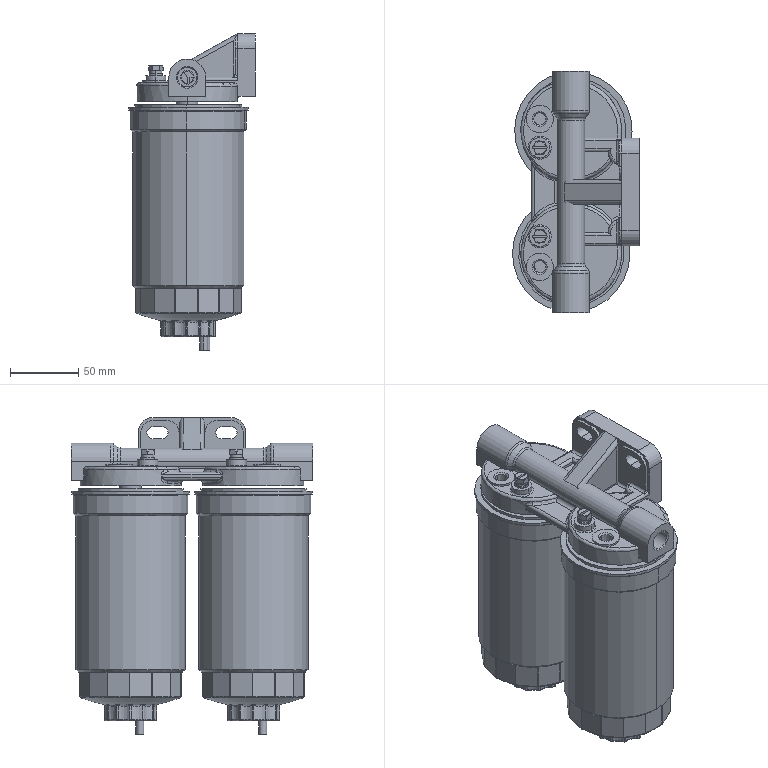Part | SolidWorks | features BaseBody 10 | 10 solids | 619 faces | box 93 x 177 x 232 mm | volume 1787680 mm3 | cylinder 217 | plane 153 | torus 96 | spline 59 | sphere 54 | cone 40 | commonest cylinder face diameters 2 x58 9 x28 18.36 x28 4 x15 20 x11 6 x8